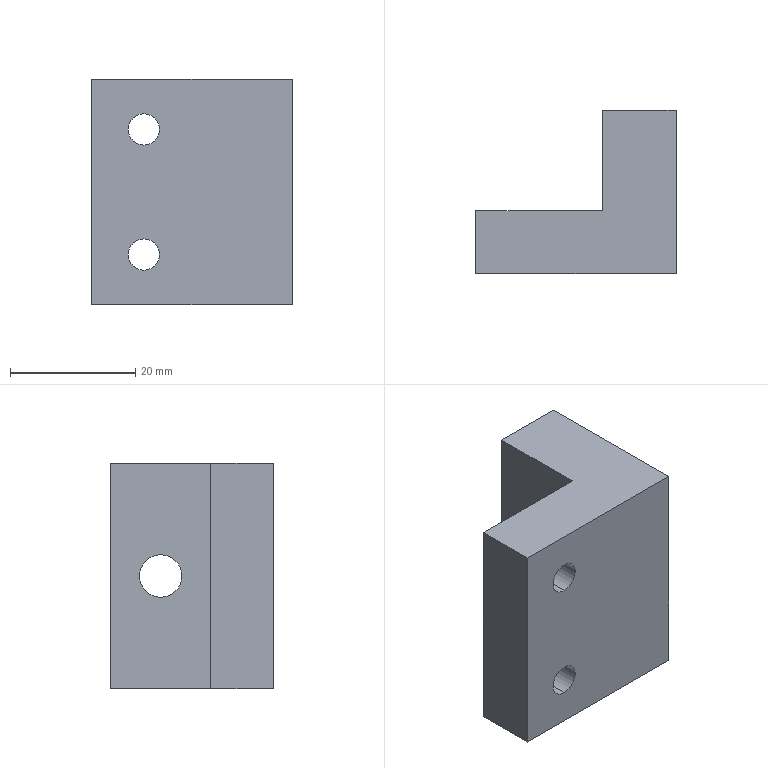Part | 1 solid | 14 faces | box 32 x 26 x 36 mm | volume 17496 mm3 | plane 8 | cylinder 6 | commonest cylinder face diameters 5 x4 6.8 x2
STEP:
#1=CARTESIAN_POINT('',(16.,18.,-3.4));
#2=VERTEX_POINT('',#1);
#3=CARTESIAN_POINT('',(16.,18.,3.4));
#4=VERTEX_POINT('',#3);
#5=CARTESIAN_POINT('',(16.,18.,0.));
#6=DIRECTION('',(-1.,0.,0.));
#7=DIRECTION('',(0.,0.,1.));
#8=AXIS2_PLACEMENT_3D('',#5,#6,#7);
#9=CIRCLE('',#8,3.4);
#10=EDGE_CURVE('',#2,#4,#9,.T.);
#11=ORIENTED_EDGE('',*,*,#10,.F.);
#12=CARTESIAN_POINT('',(4.2,18.,-3.4));
#13=VERTEX_POINT('',#12);
#14=CARTESIAN_POINT('',(4.2,18.,-3.4));
#15=DIRECTION('',(-1.,0.,0.));
#16=VECTOR('',#15,1000.);
#17=LINE('',#14,#16);
#18=EDGE_CURVE('',#2,#13,#17,.T.);
#19=ORIENTED_EDGE('',*,*,#18,.T.);
#20=CARTESIAN_POINT('',(4.2,18.,3.4));
#21=VERTEX_POINT('',#20);
#22=CARTESIAN_POINT('',(4.2,18.,0.));
#23=DIRECTION('',(-1.,0.,0.));
#24=DIRECTION('',(0.,0.,1.));
#25=AXIS2_PLACEMENT_3D('',#22,#23,#24);
#26=CIRCLE('',#25,3.4);
#27=EDGE_CURVE('',#13,#21,#26,.T.);
#28=ORIENTED_EDGE('',*,*,#27,.T.);
#29=CARTESIAN_POINT('',(4.2,18.,3.4));
#30=DIRECTION('',(-1.,0.,0.));
#31=VECTOR('',#30,1000.);
#32=LINE('',#29,#31);
#33=EDGE_CURVE('',#4,#21,#32,.T.);
#34=ORIENTED_EDGE('',*,*,#33,.F.);
#35=EDGE_LOOP('',(#11,#19,#28,#34));
#36=FACE_OUTER_BOUND('',#35,.T.);
#37=CARTESIAN_POINT('',(4.2,18.,0.));
#38=DIRECTION('',(-1.,0.,0.));
#39=DIRECTION('',(0.,0.,1.));
#40=AXIS2_PLACEMENT_3D('',#37,#38,#39);
#41=CYLINDRICAL_SURFACE('',#40,3.4);
#42=ADVANCED_FACE('',(#36),#41,.F.);
#43=CARTESIAN_POINT('',(-7.7,0.,7.5));
#44=VERTEX_POINT('',#43);
#45=CARTESIAN_POINT('',(-7.7,0.,12.5));
#46=VERTEX_POINT('',#45);
#47=CARTESIAN_POINT('',(-7.7,0.,10.));
#48=DIRECTION('',(0.,1.,0.));
#49=DIRECTION('',(0.,0.,1.));
#50=AXIS2_PLACEMENT_3D('',#47,#48,#49);
#51=CIRCLE('',#50,2.5);
#52=EDGE_CURVE('',#44,#46,#51,.T.);
#53=ORIENTED_EDGE('',*,*,#52,.F.);
#54=CARTESIAN_POINT('',(-7.7,10.,7.5));
#55=VERTEX_POINT('',#54);
#56=CARTESIAN_POINT('',(-7.7,10.,7.5));
#57=DIRECTION('',(0.,1.,0.));
#58=VECTOR('',#57,1000.);
#59=LINE('',#56,#58);
#60=EDGE_CURVE('',#44,#55,#59,.T.);
#61=ORIENTED_EDGE('',*,*,#60,.T.);
#62=CARTESIAN_POINT('',(-7.7,10.,12.5));
#63=VERTEX_POINT('',#62);
#64=CARTESIAN_POINT('',(-7.7,10.,10.));
#65=DIRECTION('',(0.,1.,0.));
#66=DIRECTION('',(0.,0.,1.));
#67=AXIS2_PLACEMENT_3D('',#64,#65,#66);
#68=CIRCLE('',#67,2.5);
#69=EDGE_CURVE('',#55,#63,#68,.T.);
#70=ORIENTED_EDGE('',*,*,#69,.T.);
#71=CARTESIAN_POINT('',(-7.7,10.,12.5));
#72=DIRECTION('',(0.,1.,0.));
#73=VECTOR('',#72,1000.);
#74=LINE('',#71,#73);
#75=EDGE_CURVE('',#46,#63,#74,.T.);
#76=ORIENTED_EDGE('',*,*,#75,.F.);
#77=EDGE_LOOP('',(#53,#61,#70,#76));
#78=FACE_OUTER_BOUND('',#77,.T.);
#79=CARTESIAN_POINT('',(-7.7,10.,10.));
#80=DIRECTION('',(0.,1.,0.));
#81=DIRECTION('',(0.,0.,1.));
#82=AXIS2_PLACEMENT_3D('',#79,#80,#81);
#83=CYLINDRICAL_SURFACE('',#82,2.5);
#84=ADVANCED_FACE('',(#78),#83,.F.);
#85=CARTESIAN_POINT('',(-7.7,0.,-12.5));
#86=VERTEX_POINT('',#85);
#87=CARTESIAN_POINT('',(-7.7,0.,-7.5));
#88=VERTEX_POINT('',#87);
#89=CARTESIAN_POINT('',(-7.7,0.,-10.));
#90=DIRECTION('',(0.,1.,0.));
#91=DIRECTION('',(0.,0.,1.));
#92=AXIS2_PLACEMENT_3D('',#89,#90,#91);
#93=CIRCLE('',#92,2.5);
#94=EDGE_CURVE('',#86,#88,#93,.T.);
#95=ORIENTED_EDGE('',*,*,#94,.F.);
#96=CARTESIAN_POINT('',(-7.7,10.,-12.5));
#97=VERTEX_POINT('',#96);
#98=CARTESIAN_POINT('',(-7.7,10.,-12.5));
#99=DIRECTION('',(0.,1.,0.));
#100=VECTOR('',#99,1000.);
#101=LINE('',#98,#100);
#102=EDGE_CURVE('',#86,#97,#101,.T.);
#103=ORIENTED_EDGE('',*,*,#102,.T.);
#104=CARTESIAN_POINT('',(-7.7,10.,-7.5));
#105=VERTEX_POINT('',#104);
#106=CARTESIAN_POINT('',(-7.7,10.,-10.));
#107=DIRECTION('',(0.,1.,0.));
#108=DIRECTION('',(0.,0.,1.));
#109=AXIS2_PLACEMENT_3D('',#106,#107,#108);
#110=CIRCLE('',#109,2.5);
#111=EDGE_CURVE('',#97,#105,#110,.T.);
#112=ORIENTED_EDGE('',*,*,#111,.T.);
#113=CARTESIAN_POINT('',(-7.7,10.,-7.5));
#114=DIRECTION('',(0.,1.,0.));
#115=VECTOR('',#114,1000.);
#116=LINE('',#113,#115);
#117=EDGE_CURVE('',#88,#105,#116,.T.);
#118=ORIENTED_EDGE('',*,*,#117,.F.);
#119=EDGE_LOOP('',(#95,#103,#112,#118));
#120=FACE_OUTER_BOUND('',#119,.T.);
#121=CARTESIAN_POINT('',(-7.7,10.,-10.));
#122=DIRECTION('',(0.,1.,0.));
#123=DIRECTION('',(0.,0.,1.));
#124=AXIS2_PLACEMENT_3D('',#121,#122,#123);
#125=CYLINDRICAL_SURFACE('',#124,2.5);
#126=ADVANCED_FACE('',(#120),#125,.F.);
#127=CARTESIAN_POINT('',(-7.7,10.,-10.));
#128=DIRECTION('',(0.,1.,0.));
#129=DIRECTION('',(0.,0.,1.));
#130=AXIS2_PLACEMENT_3D('',#127,#128,#129);
#131=CIRCLE('',#130,2.5);
#132=EDGE_CURVE('',#105,#97,#131,.T.);
#133=ORIENTED_EDGE('',*,*,#132,.F.);
#134=ORIENTED_EDGE('',*,*,#111,.F.);
#135=EDGE_LOOP('',(#133,#134));
#136=FACE_BOUND('',#135,.T.);
#137=CARTESIAN_POINT('',(-7.7,10.,10.));
#138=DIRECTION('',(0.,1.,0.));
#139=DIRECTION('',(0.,0.,1.));
#140=AXIS2_PLACEMENT_3D('',#137,#138,#139);
#141=CIRCLE('',#140,2.5);
#142=EDGE_CURVE('',#63,#55,#141,.T.);
#143=ORIENTED_EDGE('',*,*,#142,.F.);
#144=ORIENTED_EDGE('',*,*,#69,.F.);
#145=EDGE_LOOP('',(#143,#144));
#146=FACE_BOUND('',#145,.T.);
#147=CARTESIAN_POINT('',(4.2,10.,-18.));
#148=VERTEX_POINT('',#147);
#149=CARTESIAN_POINT('',(4.2,10.,18.));
#150=VERTEX_POINT('',#149);
#151=CARTESIAN_POINT('',(4.2,10.,-18.));
#152=DIRECTION('',(0.,0.,1.));
#153=VECTOR('',#152,1000.);
#154=LINE('',#151,#153);
#155=EDGE_CURVE('',#148,#150,#154,.T.);
#156=ORIENTED_EDGE('',*,*,#155,.F.);
#157=CARTESIAN_POINT('',(-16.,10.,-18.));
#158=VERTEX_POINT('',#157);
#159=CARTESIAN_POINT('',(-16.,10.,-18.));
#160=DIRECTION('',(-1.,0.,0.));
#161=VECTOR('',#160,1000.);
#162=LINE('',#159,#161);
#163=EDGE_CURVE('',#148,#158,#162,.T.);
#164=ORIENTED_EDGE('',*,*,#163,.T.);
#165=CARTESIAN_POINT('',(-16.,10.,18.));
#166=VERTEX_POINT('',#165);
#167=CARTESIAN_POINT('',(-16.,10.,18.));
#168=DIRECTION('',(0.,0.,1.));
#169=VECTOR('',#168,1000.);
#170=LINE('',#167,#169);
#171=EDGE_CURVE('',#158,#166,#170,.T.);
#172=ORIENTED_EDGE('',*,*,#171,.T.);
#173=CARTESIAN_POINT('',(-16.,10.,18.));
#174=DIRECTION('',(1.,0.,0.));
#175=VECTOR('',#174,1000.);
#176=LINE('',#173,#175);
#177=EDGE_CURVE('',#166,#150,#176,.T.);
#178=ORIENTED_EDGE('',*,*,#177,.T.);
#179=EDGE_LOOP('',(#156,#164,#172,#178));
#180=FACE_OUTER_BOUND('',#179,.T.);
#181=CARTESIAN_POINT('',(0.,10.,0.));
#182=DIRECTION('',(0.,-1.,0.));
#183=DIRECTION('',(0.,0.,-1.));
#184=AXIS2_PLACEMENT_3D('',#181,#182,#183);
#185=PLANE('',#184);
#186=ADVANCED_FACE('',(#136,#146,#180),#185,.F.);
#187=CARTESIAN_POINT('',(16.,18.,0.));
#188=DIRECTION('',(-1.,0.,0.));
#189=DIRECTION('',(0.,0.,1.));
#190=AXIS2_PLACEMENT_3D('',#187,#188,#189);
#191=CIRCLE('',#190,3.4);
#192=EDGE_CURVE('',#4,#2,#191,.T.);
#193=ORIENTED_EDGE('',*,*,#192,.T.);
#194=ORIENTED_EDGE('',*,*,#10,.T.);
#195=EDGE_LOOP('',(#193,#194));
#196=FACE_BOUND('',#195,.T.);
#197=CARTESIAN_POINT('',(16.,0.,18.));
#198=VERTEX_POINT('',#197);
#199=CARTESIAN_POINT('',(16.,0.,-18.));
#200=VERTEX_POINT('',#199);
#201=CARTESIAN_POINT('',(16.,0.,18.));
#202=DIRECTION('',(0.,0.,-1.));
#203=VECTOR('',#202,1000.);
#204=LINE('',#201,#203);
#205=EDGE_CURVE('',#198,#200,#204,.T.);
#206=ORIENTED_EDGE('',*,*,#205,.T.);
#207=CARTESIAN_POINT('',(16.,26.,-18.));
#208=VERTEX_POINT('',#207);
#209=CARTESIAN_POINT('',(16.,10.,-18.));
#210=DIRECTION('',(0.,-1.,0.));
#211=VECTOR('',#210,1000.);
#212=LINE('',#209,#211);
#213=EDGE_CURVE('',#208,#200,#212,.T.);
#214=ORIENTED_EDGE('',*,*,#213,.F.);
#215=CARTESIAN_POINT('',(16.,26.,18.));
#216=VERTEX_POINT('',#215);
#217=CARTESIAN_POINT('',(16.,26.,-18.));
#218=DIRECTION('',(0.,0.,-1.));
#219=VECTOR('',#218,1000.);
#220=LINE('',#217,#219);
#221=EDGE_CURVE('',#216,#208,#220,.T.);
#222=ORIENTED_EDGE('',*,*,#221,.F.);
#223=CARTESIAN_POINT('',(16.,10.,18.));
#224=DIRECTION('',(0.,-1.,0.));
#225=VECTOR('',#224,1000.);
#226=LINE('',#223,#225);
#227=EDGE_CURVE('',#216,#198,#226,.T.);
#228=ORIENTED_EDGE('',*,*,#227,.T.);
#229=EDGE_LOOP('',(#206,#214,#222,#228));
#230=FACE_OUTER_BOUND('',#229,.T.);
#231=CARTESIAN_POINT('',(16.,10.,18.));
#232=DIRECTION('',(-1.,0.,0.));
#233=DIRECTION('',(0.,0.,1.));
#234=AXIS2_PLACEMENT_3D('',#231,#232,#233);
#235=PLANE('',#234);
#236=ADVANCED_FACE('',(#196,#230),#235,.F.);
#237=CARTESIAN_POINT('',(-16.,0.,-18.));
#238=VERTEX_POINT('',#237);
#239=CARTESIAN_POINT('',(-16.,0.,-18.));
#240=DIRECTION('',(-1.,0.,0.));
#241=VECTOR('',#240,1000.);
#242=LINE('',#239,#241);
#243=EDGE_CURVE('',#200,#238,#242,.T.);
#244=ORIENTED_EDGE('',*,*,#243,.T.);
#245=CARTESIAN_POINT('',(-16.,10.,-18.));
#246=DIRECTION('',(0.,-1.,0.));
#247=VECTOR('',#246,1000.);
#248=LINE('',#245,#247);
#249=EDGE_CURVE('',#158,#238,#248,.T.);
#250=ORIENTED_EDGE('',*,*,#249,.F.);
#251=ORIENTED_EDGE('',*,*,#163,.F.);
#252=CARTESIAN_POINT('',(4.2,26.,-18.));
#253=VERTEX_POINT('',#252);
#254=CARTESIAN_POINT('',(4.2,26.,-18.));
#255=DIRECTION('',(0.,-1.,0.));
#256=VECTOR('',#255,1000.);
#257=LINE('',#254,#256);
#258=EDGE_CURVE('',#253,#148,#257,.T.);
#259=ORIENTED_EDGE('',*,*,#258,.F.);
#260=CARTESIAN_POINT('',(16.,26.,-18.));
#261=DIRECTION('',(-1.,0.,0.));
#262=VECTOR('',#261,1000.);
#263=LINE('',#260,#262);
#264=EDGE_CURVE('',#208,#253,#263,.T.);
#265=ORIENTED_EDGE('',*,*,#264,.F.);
#266=ORIENTED_EDGE('',*,*,#213,.T.);
#267=EDGE_LOOP('',(#244,#250,#251,#259,#265,#266));
#268=FACE_OUTER_BOUND('',#267,.T.);
#269=CARTESIAN_POINT('',(-16.,10.,-18.));
#270=DIRECTION('',(0.,0.,1.));
#271=DIRECTION('',(1.,0.,0.));
#272=AXIS2_PLACEMENT_3D('',#269,#270,#271);
#273=PLANE('',#272);
#274=ADVANCED_FACE('',(#268),#273,.F.);
#275=CARTESIAN_POINT('',(-16.,0.,18.));
#276=VERTEX_POINT('',#275);
#277=CARTESIAN_POINT('',(-16.,0.,18.));
#278=DIRECTION('',(0.,0.,1.));
#279=VECTOR('',#278,1000.);
#280=LINE('',#277,#279);
#281=EDGE_CURVE('',#238,#276,#280,.T.);
#282=ORIENTED_EDGE('',*,*,#281,.T.);
#283=CARTESIAN_POINT('',(-16.,10.,18.));
#284=DIRECTION('',(0.,-1.,0.));
#285=VECTOR('',#284,1000.);
#286=LINE('',#283,#285);
#287=EDGE_CURVE('',#166,#276,#286,.T.);
#288=ORIENTED_EDGE('',*,*,#287,.F.);
#289=ORIENTED_EDGE('',*,*,#171,.F.);
#290=ORIENTED_EDGE('',*,*,#249,.T.);
#291=EDGE_LOOP('',(#282,#288,#289,#290));
#292=FACE_OUTER_BOUND('',#291,.T.);
#293=CARTESIAN_POINT('',(-16.,10.,18.));
#294=DIRECTION('',(1.,0.,0.));
#295=DIRECTION('',(0.,0.,-1.));
#296=AXIS2_PLACEMENT_3D('',#293,#294,#295);
#297=PLANE('',#296);
#298=ADVANCED_FACE('',(#292),#297,.F.);
#299=CARTESIAN_POINT('',(-16.,0.,18.));
#300=DIRECTION('',(1.,0.,0.));
#301=VECTOR('',#300,1000.);
#302=LINE('',#299,#301);
#303=EDGE_CURVE('',#276,#198,#302,.T.);
#304=ORIENTED_EDGE('',*,*,#303,.T.);
#305=ORIENTED_EDGE('',*,*,#227,.F.);
#306=CARTESIAN_POINT('',(4.2,26.,18.));
#307=VERTEX_POINT('',#306);
#308=CARTESIAN_POINT('',(16.,26.,18.));
#309=DIRECTION('',(1.,0.,0.));
#310=VECTOR('',#309,1000.);
#311=LINE('',#308,#310);
#312=EDGE_CURVE('',#307,#216,#311,.T.);
#313=ORIENTED_EDGE('',*,*,#312,.F.);
#314=CARTESIAN_POINT('',(4.2,26.,18.));
#315=DIRECTION('',(0.,-1.,0.));
#316=VECTOR('',#315,1000.);
#317=LINE('',#314,#316);
#318=EDGE_CURVE('',#307,#150,#317,.T.);
#319=ORIENTED_EDGE('',*,*,#318,.T.);
#320=ORIENTED_EDGE('',*,*,#177,.F.);
#321=ORIENTED_EDGE('',*,*,#287,.T.);
#322=EDGE_LOOP('',(#304,#305,#313,#319,#320,#321));
#323=FACE_OUTER_BOUND('',#322,.T.);
#324=CARTESIAN_POINT('',(-16.,10.,18.));
#325=DIRECTION('',(0.,0.,-1.));
#326=DIRECTION('',(-1.,0.,0.));
#327=AXIS2_PLACEMENT_3D('',#324,#325,#326);
#328=PLANE('',#327);
#329=ADVANCED_FACE('',(#323),#328,.F.);
#330=CARTESIAN_POINT('',(-7.7,0.,10.));
#331=DIRECTION('',(0.,1.,0.));
#332=DIRECTION('',(0.,0.,1.));
#333=AXIS2_PLACEMENT_3D('',#330,#331,#332);
#334=CIRCLE('',#333,2.5);
#335=EDGE_CURVE('',#46,#44,#334,.T.);
#336=ORIENTED_EDGE('',*,*,#335,.T.);
#337=ORIENTED_EDGE('',*,*,#52,.T.);
#338=EDGE_LOOP('',(#336,#337));
#339=FACE_BOUND('',#338,.T.);
#340=CARTESIAN_POINT('',(-7.7,0.,-10.));
#341=DIRECTION('',(0.,1.,0.));
#342=DIRECTION('',(0.,0.,1.));
#343=AXIS2_PLACEMENT_3D('',#340,#341,#342);
#344=CIRCLE('',#343,2.5);
#345=EDGE_CURVE('',#88,#86,#344,.T.);
#346=ORIENTED_EDGE('',*,*,#345,.T.);
#347=ORIENTED_EDGE('',*,*,#94,.T.);
#348=EDGE_LOOP('',(#346,#347));
#349=FACE_BOUND('',#348,.T.);
#350=ORIENTED_EDGE('',*,*,#205,.F.);
#351=ORIENTED_EDGE('',*,*,#303,.F.);
#352=ORIENTED_EDGE('',*,*,#281,.F.);
#353=ORIENTED_EDGE('',*,*,#243,.F.);
#354=EDGE_LOOP('',(#350,#351,#352,#353));
#355=FACE_OUTER_BOUND('',#354,.T.);
#356=CARTESIAN_POINT('',(0.,0.,0.));
#357=DIRECTION('',(0.,-1.,0.));
#358=DIRECTION('',(0.,0.,-1.));
#359=AXIS2_PLACEMENT_3D('',#356,#357,#358);
#360=PLANE('',#359);
#361=ADVANCED_FACE('',(#339,#349,#355),#360,.T.);
#362=ORIENTED_EDGE('',*,*,#102,.F.);
#363=ORIENTED_EDGE('',*,*,#345,.F.);
#364=ORIENTED_EDGE('',*,*,#117,.T.);
#365=ORIENTED_EDGE('',*,*,#132,.T.);
#366=EDGE_LOOP('',(#362,#363,#364,#365));
#367=FACE_OUTER_BOUND('',#366,.T.);
#368=CARTESIAN_POINT('',(-7.7,10.,-10.));
#369=DIRECTION('',(0.,1.,0.));
#370=DIRECTION('',(0.,0.,1.));
#371=AXIS2_PLACEMENT_3D('',#368,#369,#370);
#372=CYLINDRICAL_SURFACE('',#371,2.5);
#373=ADVANCED_FACE('',(#367),#372,.F.);
#374=ORIENTED_EDGE('',*,*,#60,.F.);
#375=ORIENTED_EDGE('',*,*,#335,.F.);
#376=ORIENTED_EDGE('',*,*,#75,.T.);
#377=ORIENTED_EDGE('',*,*,#142,.T.);
#378=EDGE_LOOP('',(#374,#375,#376,#377));
#379=FACE_OUTER_BOUND('',#378,.T.);
#380=CARTESIAN_POINT('',(-7.7,10.,10.));
#381=DIRECTION('',(0.,1.,0.));
#382=DIRECTION('',(0.,0.,1.));
#383=AXIS2_PLACEMENT_3D('',#380,#381,#382);
#384=CYLINDRICAL_SURFACE('',#383,2.5);
#385=ADVANCED_FACE('',(#379),#384,.F.);
#386=CARTESIAN_POINT('',(4.2,18.,0.));
#387=DIRECTION('',(-1.,0.,0.));
#388=DIRECTION('',(0.,0.,1.));
#389=AXIS2_PLACEMENT_3D('',#386,#387,#388);
#390=CIRCLE('',#389,3.4);
#391=EDGE_CURVE('',#21,#13,#390,.T.);
#392=ORIENTED_EDGE('',*,*,#391,.F.);
#393=ORIENTED_EDGE('',*,*,#27,.F.);
#394=EDGE_LOOP('',(#392,#393));
#395=FACE_BOUND('',#394,.T.);
#396=ORIENTED_EDGE('',*,*,#155,.T.);
#397=ORIENTED_EDGE('',*,*,#318,.F.);
#398=CARTESIAN_POINT('',(4.2,26.,-18.));
#399=DIRECTION('',(0.,0.,1.));
#400=VECTOR('',#399,1000.);
#401=LINE('',#398,#400);
#402=EDGE_CURVE('',#253,#307,#401,.T.);
#403=ORIENTED_EDGE('',*,*,#402,.F.);
#404=ORIENTED_EDGE('',*,*,#258,.T.);
#405=EDGE_LOOP('',(#396,#397,#403,#404));
#406=FACE_OUTER_BOUND('',#405,.T.);
#407=CARTESIAN_POINT('',(4.2,26.,-18.));
#408=DIRECTION('',(1.,0.,0.));
#409=DIRECTION('',(0.,0.,-1.));
#410=AXIS2_PLACEMENT_3D('',#407,#408,#409);
#411=PLANE('',#410);
#412=ADVANCED_FACE('',(#395,#406),#411,.F.);
#413=ORIENTED_EDGE('',*,*,#221,.T.);
#414=ORIENTED_EDGE('',*,*,#264,.T.);
#415=ORIENTED_EDGE('',*,*,#402,.T.);
#416=ORIENTED_EDGE('',*,*,#312,.T.);
#417=EDGE_LOOP('',(#413,#414,#415,#416));
#418=FACE_OUTER_BOUND('',#417,.T.);
#419=CARTESIAN_POINT('',(0.,26.,0.));
#420=DIRECTION('',(0.,-1.,0.));
#421=DIRECTION('',(0.,0.,-1.));
#422=AXIS2_PLACEMENT_3D('',#419,#420,#421);
#423=PLANE('',#422);
#424=ADVANCED_FACE('',(#418),#423,.F.);
#425=ORIENTED_EDGE('',*,*,#18,.F.);
#426=ORIENTED_EDGE('',*,*,#192,.F.);
#427=ORIENTED_EDGE('',*,*,#33,.T.);
#428=ORIENTED_EDGE('',*,*,#391,.T.);
#429=EDGE_LOOP('',(#425,#426,#427,#428));
#430=FACE_OUTER_BOUND('',#429,.T.);
#431=CARTESIAN_POINT('',(4.2,18.,0.));
#432=DIRECTION('',(-1.,0.,0.));
#433=DIRECTION('',(0.,0.,1.));
#434=AXIS2_PLACEMENT_3D('',#431,#432,#433);
#435=CYLINDRICAL_SURFACE('',#434,3.4);
#436=ADVANCED_FACE('',(#430),#435,.F.);
#437=CLOSED_SHELL('',(#42,#84,#126,#186,#236,#274,#298,#329,#361,#373,#385,#412,#424,#436));
#438=MANIFOLD_SOLID_BREP('',#437);
#439=CARTESIAN_POINT('',(0.,0.,0.));
#440=DIRECTION('',(0.,0.,1.));
#441=DIRECTION('',(1.,0.,0.));
#442=AXIS2_PLACEMENT_3D('',#439,#440,#441);
#443=(LENGTH_UNIT()NAMED_UNIT(*)SI_UNIT(.MILLI.,.METRE.));
#444=UNCERTAINTY_MEASURE_WITH_UNIT(LENGTH_MEASURE(0.00001),#443,'','');
#445=(NAMED_UNIT(*)PLANE_ANGLE_UNIT()SI_UNIT($,.RADIAN.));
#446=(NAMED_UNIT(*)SI_UNIT($,.STERADIAN.)SOLID_ANGLE_UNIT());
#447=(GEOMETRIC_REPRESENTATION_CONTEXT(3)GLOBAL_UNCERTAINTY_ASSIGNED_CONTEXT((#444))GLOBAL_UNIT_ASSIGNED_CONTEXT((#443,#445,#446))REPRESENTATION_CONTEXT('',''));
#448=ADVANCED_BREP_SHAPE_REPRESENTATION('',(#438,#442),#447);